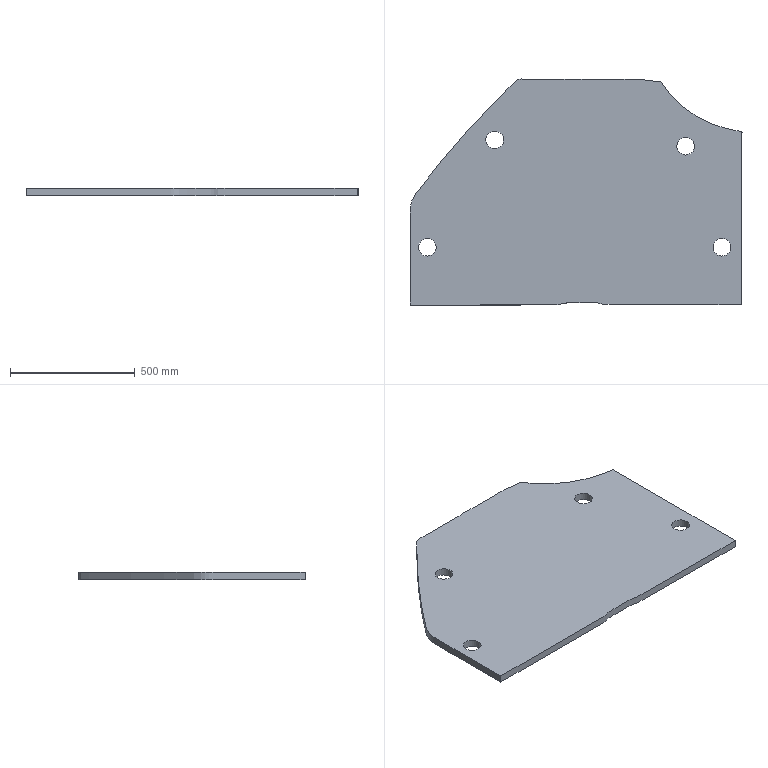Part | NX | features solid 2 | 1 solid | 10 faces | box 1330 x 905.627 x 30 mm | volume 31286840 mm3 | spline 4 | cylinder 4 | plane 2 | commonest cylinder face diameters 71 x4